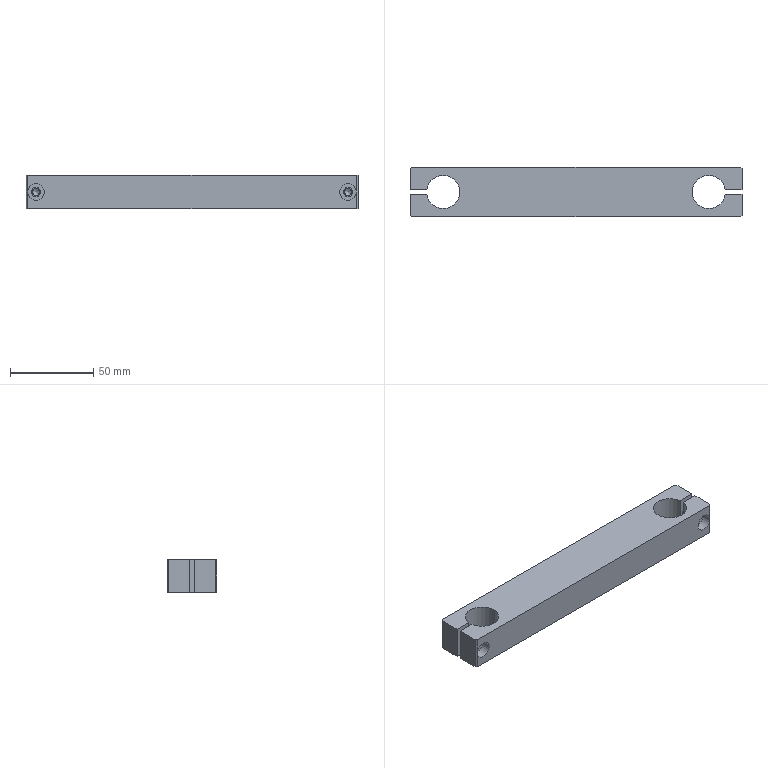Part | NX | features B0002 2 | 1 solid | 30 faces | box 200 x 30 x 20 mm | volume 103319 mm3 | plane 18 | cylinder 9 | cone 3 | commonest cylinder face diameters 4.2 x2 5.5 x2 10 x2 20 x2 8.5 x1
STEP:
#1=CARTESIAN_POINT('',(-94.,15.7,-379.25));
#2=VERTEX_POINT('',#1);
#3=CARTESIAN_POINT('',(-94.,15.7,-382.));
#4=DIRECTION('',(0.,1.,0.));
#5=DIRECTION('',(0.,0.,1.));
#6=AXIS2_PLACEMENT_3D('',#3,#4,#5);
#7=CIRCLE('',#6,2.75);
#8=EDGE_CURVE('',#2,#2,#7,.T.);
#9=ORIENTED_EDGE('',*,*,#8,.T.);
#10=EDGE_LOOP('',(#9));
#11=FACE_BOUND('',#10,.T.);
#12=CARTESIAN_POINT('',(-94.,15.7,-377.));
#13=VERTEX_POINT('',#12);
#14=CARTESIAN_POINT('',(-94.,15.7,-382.));
#15=DIRECTION('',(0.,-1.,0.));
#16=DIRECTION('',(0.,0.,1.));
#17=AXIS2_PLACEMENT_3D('',#14,#15,#16);
#18=CIRCLE('',#17,5.);
#19=EDGE_CURVE('',#13,#13,#18,.T.);
#20=ORIENTED_EDGE('',*,*,#19,.T.);
#21=EDGE_LOOP('',(#20));
#22=FACE_BOUND('',#21,.T.);
#23=CARTESIAN_POINT('',(-96.75,15.7,-382.));
#24=DIRECTION('',(0.,1.,0.));
#25=DIRECTION('',(0.,0.,-1.));
#26=AXIS2_PLACEMENT_3D('',#23,#24,#25);
#27=PLANE('',#26);
#28=ADVANCED_FACE('',(#11,#22),#27,.F.);
#29=CARTESIAN_POINT('',(-99.,10.,-382.));
#30=VERTEX_POINT('',#29);
#31=CARTESIAN_POINT('',(-94.,10.,-382.));
#32=DIRECTION('',(0.,1.,0.));
#33=DIRECTION('',(0.,0.,-1.));
#34=AXIS2_PLACEMENT_3D('',#31,#32,#33);
#35=CIRCLE('',#34,5.);
#36=EDGE_CURVE('',#30,#30,#35,.T.);
#37=ORIENTED_EDGE('',*,*,#36,.F.);
#38=EDGE_LOOP('',(#37));
#39=FACE_BOUND('',#38,.T.);
#40=ORIENTED_EDGE('',*,*,#19,.F.);
#41=EDGE_LOOP('',(#40));
#42=FACE_BOUND('',#41,.T.);
#43=CARTESIAN_POINT('',(-94.,10.,-382.));
#44=DIRECTION('',(0.,-1.,0.));
#45=DIRECTION('',(0.,0.,1.));
#46=AXIS2_PLACEMENT_3D('',#43,#44,#45);
#47=CYLINDRICAL_SURFACE('',#46,5.);
#48=ADVANCED_FACE('',(#39,#42),#47,.F.);
#49=CARTESIAN_POINT('',(99.,10.,-382.));
#50=VERTEX_POINT('',#49);
#51=CARTESIAN_POINT('',(94.,10.,-382.));
#52=DIRECTION('',(0.,1.,0.));
#53=DIRECTION('',(0.,0.,1.));
#54=AXIS2_PLACEMENT_3D('',#51,#52,#53);
#55=CIRCLE('',#54,5.);
#56=EDGE_CURVE('',#50,#50,#55,.T.);
#57=ORIENTED_EDGE('',*,*,#56,.F.);
#58=EDGE_LOOP('',(#57));
#59=FACE_BOUND('',#58,.T.);
#60=CARTESIAN_POINT('',(94.,15.7,-377.));
#61=VERTEX_POINT('',#60);
#62=CARTESIAN_POINT('',(94.,15.7,-382.));
#63=DIRECTION('',(0.,-1.,0.));
#64=DIRECTION('',(0.,0.,1.));
#65=AXIS2_PLACEMENT_3D('',#62,#63,#64);
#66=CIRCLE('',#65,5.);
#67=EDGE_CURVE('',#61,#61,#66,.T.);
#68=ORIENTED_EDGE('',*,*,#67,.F.);
#69=EDGE_LOOP('',(#68));
#70=FACE_BOUND('',#69,.T.);
#71=CARTESIAN_POINT('',(94.,10.,-382.));
#72=DIRECTION('',(0.,-1.,0.));
#73=DIRECTION('',(0.,0.,1.));
#74=AXIS2_PLACEMENT_3D('',#71,#72,#73);
#75=CYLINDRICAL_SURFACE('',#74,5.);
#76=ADVANCED_FACE('',(#59,#70),#75,.F.);
#77=CARTESIAN_POINT('',(94.,15.7,-384.75));
#78=VERTEX_POINT('',#77);
#79=CARTESIAN_POINT('',(94.,15.7,-382.));
#80=DIRECTION('',(0.,1.,0.));
#81=DIRECTION('',(0.,0.,-1.));
#82=AXIS2_PLACEMENT_3D('',#79,#80,#81);
#83=CIRCLE('',#82,2.75);
#84=EDGE_CURVE('',#78,#78,#83,.T.);
#85=ORIENTED_EDGE('',*,*,#84,.T.);
#86=EDGE_LOOP('',(#85));
#87=FACE_BOUND('',#86,.T.);
#88=ORIENTED_EDGE('',*,*,#67,.T.);
#89=EDGE_LOOP('',(#88));
#90=FACE_BOUND('',#89,.T.);
#91=CARTESIAN_POINT('',(91.25,15.7,-382.));
#92=DIRECTION('',(0.,1.,0.));
#93=DIRECTION('',(0.,0.,-1.));
#94=AXIS2_PLACEMENT_3D('',#91,#92,#93);
#95=PLANE('',#94);
#96=ADVANCED_FACE('',(#87,#90),#95,.F.);
#97=CARTESIAN_POINT('',(94.,23.75,-379.25));
#98=VERTEX_POINT('',#97);
#99=CARTESIAN_POINT('',(94.,23.75,-382.));
#100=DIRECTION('',(0.,-1.,0.));
#101=DIRECTION('',(0.,0.,1.));
#102=AXIS2_PLACEMENT_3D('',#99,#100,#101);
#103=CIRCLE('',#102,2.75);
#104=EDGE_CURVE('',#98,#98,#103,.T.);
#105=ORIENTED_EDGE('',*,*,#104,.F.);
#106=EDGE_LOOP('',(#105));
#107=FACE_BOUND('',#106,.T.);
#108=ORIENTED_EDGE('',*,*,#84,.F.);
#109=EDGE_LOOP('',(#108));
#110=FACE_BOUND('',#109,.T.);
#111=CARTESIAN_POINT('',(94.,10.,-382.));
#112=DIRECTION('',(0.,-1.,0.));
#113=DIRECTION('',(0.,0.,1.));
#114=AXIS2_PLACEMENT_3D('',#111,#112,#113);
#115=CYLINDRICAL_SURFACE('',#114,2.75);
#116=ADVANCED_FACE('',(#107,#110),#115,.F.);
#117=CARTESIAN_POINT('',(94.,38.65,-379.9));
#118=VERTEX_POINT('',#117);
#119=CARTESIAN_POINT('',(94.,38.65,-382.));
#120=DIRECTION('',(0.,-1.,0.));
#121=DIRECTION('',(0.,0.,1.));
#122=AXIS2_PLACEMENT_3D('',#119,#120,#121);
#123=CIRCLE('',#122,2.1);
#124=EDGE_CURVE('',#118,#118,#123,.T.);
#125=ORIENTED_EDGE('',*,*,#124,.T.);
#126=EDGE_LOOP('',(#125));
#127=FACE_BOUND('',#126,.T.);
#128=CARTESIAN_POINT('',(94.,39.912,-382.));
#129=VERTEX_POINT('',#128);
#130=VERTEX_LOOP('',#129);
#131=FACE_BOUND('',#130,.T.);
#132=CARTESIAN_POINT('',(94.,39.912,-382.));
#133=DIRECTION('',(0.,-1.,0.));
#134=DIRECTION('',(0.,0.,1.));
#135=AXIS2_PLACEMENT_3D('',#132,#133,#134);
#136=CONICAL_SURFACE('',#135,0.,1.03);
#137=ADVANCED_FACE('',(#127,#131),#136,.F.);
#138=CARTESIAN_POINT('',(94.,26.25,-384.1));
#139=VERTEX_POINT('',#138);
#140=CARTESIAN_POINT('',(94.,26.25,-382.));
#141=DIRECTION('',(0.,1.,0.));
#142=DIRECTION('',(0.,0.,-1.));
#143=AXIS2_PLACEMENT_3D('',#140,#141,#142);
#144=CIRCLE('',#143,2.1);
#145=EDGE_CURVE('',#139,#139,#144,.T.);
#146=ORIENTED_EDGE('',*,*,#145,.F.);
#147=EDGE_LOOP('',(#146));
#148=FACE_BOUND('',#147,.T.);
#149=ORIENTED_EDGE('',*,*,#124,.F.);
#150=EDGE_LOOP('',(#149));
#151=FACE_BOUND('',#150,.T.);
#152=CARTESIAN_POINT('',(94.,26.25,-382.));
#153=DIRECTION('',(0.,-1.,0.));
#154=DIRECTION('',(0.,0.,1.));
#155=AXIS2_PLACEMENT_3D('',#152,#153,#154);
#156=CYLINDRICAL_SURFACE('',#155,2.1);
#157=ADVANCED_FACE('',(#148,#151),#156,.F.);
#158=CARTESIAN_POINT('',(0.,12.946,-382.));
#159=VERTEX_POINT('',#158);
#160=VERTEX_LOOP('',#159);
#161=FACE_BOUND('',#160,.T.);
#162=CARTESIAN_POINT('',(0.,15.5,-386.25));
#163=VERTEX_POINT('',#162);
#164=CARTESIAN_POINT('',(0.,15.5,-382.));
#165=DIRECTION('',(0.,1.,0.));
#166=DIRECTION('',(0.,0.,-1.));
#167=AXIS2_PLACEMENT_3D('',#164,#165,#166);
#168=CIRCLE('',#167,4.25);
#169=EDGE_CURVE('',#163,#163,#168,.T.);
#170=ORIENTED_EDGE('',*,*,#169,.T.);
#171=EDGE_LOOP('',(#170));
#172=FACE_BOUND('',#171,.T.);
#173=CARTESIAN_POINT('',(0.,12.946,-382.));
#174=DIRECTION('',(0.,1.,0.));
#175=DIRECTION('',(0.,0.,-1.));
#176=AXIS2_PLACEMENT_3D('',#173,#174,#175);
#177=CONICAL_SURFACE('',#176,0.,1.03);
#178=ADVANCED_FACE('',(#161,#172),#177,.F.);
#179=ORIENTED_EDGE('',*,*,#169,.F.);
#180=EDGE_LOOP('',(#179));
#181=FACE_BOUND('',#180,.T.);
#182=CARTESIAN_POINT('',(0.,40.,-377.75));
#183=VERTEX_POINT('',#182);
#184=CARTESIAN_POINT('',(0.,40.,-382.));
#185=DIRECTION('',(0.,-1.,0.));
#186=DIRECTION('',(0.,0.,1.));
#187=AXIS2_PLACEMENT_3D('',#184,#185,#186);
#188=CIRCLE('',#187,4.25);
#189=EDGE_CURVE('',#183,#183,#188,.T.);
#190=ORIENTED_EDGE('',*,*,#189,.F.);
#191=EDGE_LOOP('',(#190));
#192=FACE_BOUND('',#191,.T.);
#193=CARTESIAN_POINT('',(0.,40.,-382.));
#194=DIRECTION('',(0.,1.,0.));
#195=DIRECTION('',(0.,0.,-1.));
#196=AXIS2_PLACEMENT_3D('',#193,#194,#195);
#197=CYLINDRICAL_SURFACE('',#196,4.25);
#198=ADVANCED_FACE('',(#181,#192),#197,.F.);
#199=CARTESIAN_POINT('',(-94.,38.65,-379.9));
#200=VERTEX_POINT('',#199);
#201=CARTESIAN_POINT('',(-94.,38.65,-382.));
#202=DIRECTION('',(0.,-1.,0.));
#203=DIRECTION('',(0.,0.,1.));
#204=AXIS2_PLACEMENT_3D('',#201,#202,#203);
#205=CIRCLE('',#204,2.1);
#206=EDGE_CURVE('',#200,#200,#205,.T.);
#207=ORIENTED_EDGE('',*,*,#206,.T.);
#208=EDGE_LOOP('',(#207));
#209=FACE_BOUND('',#208,.T.);
#210=CARTESIAN_POINT('',(-94.,39.912,-382.));
#211=VERTEX_POINT('',#210);
#212=VERTEX_LOOP('',#211);
#213=FACE_BOUND('',#212,.T.);
#214=CARTESIAN_POINT('',(-94.,39.912,-382.));
#215=DIRECTION('',(0.,-1.,0.));
#216=DIRECTION('',(0.,0.,1.));
#217=AXIS2_PLACEMENT_3D('',#214,#215,#216);
#218=CONICAL_SURFACE('',#217,0.,1.03);
#219=ADVANCED_FACE('',(#209,#213),#218,.F.);
#220=ORIENTED_EDGE('',*,*,#206,.F.);
#221=EDGE_LOOP('',(#220));
#222=FACE_BOUND('',#221,.T.);
#223=CARTESIAN_POINT('',(-94.,26.25,-384.1));
#224=VERTEX_POINT('',#223);
#225=CARTESIAN_POINT('',(-94.,26.25,-382.));
#226=DIRECTION('',(0.,1.,0.));
#227=DIRECTION('',(0.,0.,-1.));
#228=AXIS2_PLACEMENT_3D('',#225,#226,#227);
#229=CIRCLE('',#228,2.1);
#230=EDGE_CURVE('',#224,#224,#229,.T.);
#231=ORIENTED_EDGE('',*,*,#230,.F.);
#232=EDGE_LOOP('',(#231));
#233=FACE_BOUND('',#232,.T.);
#234=CARTESIAN_POINT('',(-94.,26.25,-382.));
#235=DIRECTION('',(0.,-1.,0.));
#236=DIRECTION('',(0.,0.,1.));
#237=AXIS2_PLACEMENT_3D('',#234,#235,#236);
#238=CYLINDRICAL_SURFACE('',#237,2.1);
#239=ADVANCED_FACE('',(#222,#233),#238,.F.);
#240=ORIENTED_EDGE('',*,*,#230,.T.);
#241=EDGE_LOOP('',(#240));
#242=FACE_BOUND('',#241,.T.);
#243=CARTESIAN_POINT('',(-89.922,26.25,-372.));
#244=VERTEX_POINT('',#243);
#245=CARTESIAN_POINT('',(-89.922,26.25,-392.));
#246=VERTEX_POINT('',#245);
#247=CARTESIAN_POINT('',(-89.922,26.25,-372.));
#248=DIRECTION('',(0.,0.,-1.));
#249=VECTOR('',#248,1000.);
#250=LINE('',#247,#249);
#251=EDGE_CURVE('',#244,#246,#250,.T.);
#252=ORIENTED_EDGE('',*,*,#251,.F.);
#253=CARTESIAN_POINT('',(-100.,26.25,-372.));
#254=VERTEX_POINT('',#253);
#255=CARTESIAN_POINT('',(-100.,26.25,-372.));
#256=DIRECTION('',(1.,0.,0.));
#257=VECTOR('',#256,1000.);
#258=LINE('',#255,#257);
#259=EDGE_CURVE('',#254,#244,#258,.T.);
#260=ORIENTED_EDGE('',*,*,#259,.F.);
#261=CARTESIAN_POINT('',(-100.,26.25,-392.));
#262=VERTEX_POINT('',#261);
#263=CARTESIAN_POINT('',(-100.,26.25,-372.));
#264=DIRECTION('',(0.,0.,-1.));
#265=VECTOR('',#264,1000.);
#266=LINE('',#263,#265);
#267=EDGE_CURVE('',#254,#262,#266,.T.);
#268=ORIENTED_EDGE('',*,*,#267,.T.);
#269=CARTESIAN_POINT('',(-89.922,26.25,-392.));
#270=DIRECTION('',(-1.,0.,0.));
#271=VECTOR('',#270,1000.);
#272=LINE('',#269,#271);
#273=EDGE_CURVE('',#246,#262,#272,.T.);
#274=ORIENTED_EDGE('',*,*,#273,.F.);
#275=EDGE_LOOP('',(#252,#260,#268,#274));
#276=FACE_BOUND('',#275,.T.);
#277=CARTESIAN_POINT('',(-80.,26.25,-392.001));
#278=DIRECTION('',(0.,1.,0.));
#279=DIRECTION('',(-1.,0.,0.));
#280=AXIS2_PLACEMENT_3D('',#277,#278,#279);
#281=PLANE('',#280);
#282=ADVANCED_FACE('',(#242,#276),#281,.F.);
#283=ORIENTED_EDGE('',*,*,#267,.F.);
#284=CARTESIAN_POINT('',(-100.,39.,-372.));
#285=VERTEX_POINT('',#284);
#286=CARTESIAN_POINT('',(-100.,26.25,-372.));
#287=DIRECTION('',(0.,1.,0.));
#288=VECTOR('',#287,1000.);
#289=LINE('',#286,#288);
#290=EDGE_CURVE('',#254,#285,#289,.T.);
#291=ORIENTED_EDGE('',*,*,#290,.T.);
#292=CARTESIAN_POINT('',(-100.,39.,-392.));
#293=VERTEX_POINT('',#292);
#294=CARTESIAN_POINT('',(-100.,39.,-392.));
#295=DIRECTION('',(0.,0.,1.));
#296=VECTOR('',#295,1000.);
#297=LINE('',#294,#296);
#298=EDGE_CURVE('',#293,#285,#297,.T.);
#299=ORIENTED_EDGE('',*,*,#298,.F.);
#300=CARTESIAN_POINT('',(-100.,26.25,-392.));
#301=DIRECTION('',(0.,1.,0.));
#302=VECTOR('',#301,1000.);
#303=LINE('',#300,#302);
#304=EDGE_CURVE('',#262,#293,#303,.T.);
#305=ORIENTED_EDGE('',*,*,#304,.F.);
#306=EDGE_LOOP('',(#283,#291,#299,#305));
#307=FACE_BOUND('',#306,.T.);
#308=CARTESIAN_POINT('',(-100.,40.,-372.));
#309=DIRECTION('',(1.,0.,0.));
#310=DIRECTION('',(0.,0.,1.));
#311=AXIS2_PLACEMENT_3D('',#308,#309,#310);
#312=PLANE('',#311);
#313=ADVANCED_FACE('',(#307),#312,.F.);
#314=CARTESIAN_POINT('',(-99.,40.,-372.));
#315=VERTEX_POINT('',#314);
#316=CARTESIAN_POINT('',(-99.,40.,-392.));
#317=VERTEX_POINT('',#316);
#318=CARTESIAN_POINT('',(-99.,40.,-372.));
#319=DIRECTION('',(0.,0.,-1.));
#320=VECTOR('',#319,1000.);
#321=LINE('',#318,#320);
#322=EDGE_CURVE('',#315,#317,#321,.T.);
#323=ORIENTED_EDGE('',*,*,#322,.T.);
#324=CARTESIAN_POINT('',(-100.,39.,-392.));
#325=DIRECTION('',(0.7071,0.7071,0.));
#326=VECTOR('',#325,1000.);
#327=LINE('',#324,#326);
#328=EDGE_CURVE('',#293,#317,#327,.T.);
#329=ORIENTED_EDGE('',*,*,#328,.F.);
#330=ORIENTED_EDGE('',*,*,#298,.T.);
#331=CARTESIAN_POINT('',(-99.,40.,-372.));
#332=DIRECTION('',(-0.7071,-0.7071,0.));
#333=VECTOR('',#332,1000.);
#334=LINE('',#331,#333);
#335=EDGE_CURVE('',#315,#285,#334,.T.);
#336=ORIENTED_EDGE('',*,*,#335,.F.);
#337=EDGE_LOOP('',(#323,#329,#330,#336));
#338=FACE_BOUND('',#337,.T.);
#339=CARTESIAN_POINT('',(-100.,39.,-372.));
#340=DIRECTION('',(0.7071,-0.7071,0.));
#341=DIRECTION('',(0.,0.,-1.));
#342=AXIS2_PLACEMENT_3D('',#339,#340,#341);
#343=PLANE('',#342);
#344=ADVANCED_FACE('',(#338),#343,.F.);
#345=ORIENTED_EDGE('',*,*,#189,.T.);
#346=EDGE_LOOP('',(#345));
#347=FACE_BOUND('',#346,.T.);
#348=ORIENTED_EDGE('',*,*,#322,.F.);
#349=CARTESIAN_POINT('',(99.,40.,-372.));
#350=VERTEX_POINT('',#349);
#351=CARTESIAN_POINT('',(-99.,40.,-372.));
#352=DIRECTION('',(1.,0.,0.));
#353=VECTOR('',#352,1000.);
#354=LINE('',#351,#353);
#355=EDGE_CURVE('',#315,#350,#354,.T.);
#356=ORIENTED_EDGE('',*,*,#355,.T.);
#357=CARTESIAN_POINT('',(99.,40.,-392.));
#358=VERTEX_POINT('',#357);
#359=CARTESIAN_POINT('',(99.,40.,-392.));
#360=DIRECTION('',(0.,0.,1.));
#361=VECTOR('',#360,1000.);
#362=LINE('',#359,#361);
#363=EDGE_CURVE('',#358,#350,#362,.T.);
#364=ORIENTED_EDGE('',*,*,#363,.F.);
#365=CARTESIAN_POINT('',(-99.,40.,-392.));
#366=DIRECTION('',(1.,0.,0.));
#367=VECTOR('',#366,1000.);
#368=LINE('',#365,#367);
#369=EDGE_CURVE('',#317,#358,#368,.T.);
#370=ORIENTED_EDGE('',*,*,#369,.F.);
#371=EDGE_LOOP('',(#348,#356,#364,#370));
#372=FACE_BOUND('',#371,.T.);
#373=CARTESIAN_POINT('',(-100.,40.,-372.));
#374=DIRECTION('',(0.,-1.,0.));
#375=DIRECTION('',(1.,0.,0.));
#376=AXIS2_PLACEMENT_3D('',#373,#374,#375);
#377=PLANE('',#376);
#378=ADVANCED_FACE('',(#347,#372),#377,.F.);
#379=CARTESIAN_POINT('',(100.,39.,-372.));
#380=VERTEX_POINT('',#379);
#381=CARTESIAN_POINT('',(100.,39.,-392.));
#382=VERTEX_POINT('',#381);
#383=CARTESIAN_POINT('',(100.,39.,-372.));
#384=DIRECTION('',(0.,0.,-1.));
#385=VECTOR('',#384,1000.);
#386=LINE('',#383,#385);
#387=EDGE_CURVE('',#380,#382,#386,.T.);
#388=ORIENTED_EDGE('',*,*,#387,.T.);
#389=CARTESIAN_POINT('',(99.,40.,-392.));
#390=DIRECTION('',(0.7071,-0.7071,0.));
#391=VECTOR('',#390,1000.);
#392=LINE('',#389,#391);
#393=EDGE_CURVE('',#358,#382,#392,.T.);
#394=ORIENTED_EDGE('',*,*,#393,.F.);
#395=ORIENTED_EDGE('',*,*,#363,.T.);
#396=CARTESIAN_POINT('',(100.,39.,-372.));
#397=DIRECTION('',(-0.7071,0.7071,0.));
#398=VECTOR('',#397,1000.);
#399=LINE('',#396,#398);
#400=EDGE_CURVE('',#380,#350,#399,.T.);
#401=ORIENTED_EDGE('',*,*,#400,.F.);
#402=EDGE_LOOP('',(#388,#394,#395,#401));
#403=FACE_BOUND('',#402,.T.);
#404=CARTESIAN_POINT('',(99.,40.,-372.));
#405=DIRECTION('',(-0.7071,-0.7071,0.));
#406=DIRECTION('',(0.,0.,-1.));
#407=AXIS2_PLACEMENT_3D('',#404,#405,#406);
#408=PLANE('',#407);
#409=ADVANCED_FACE('',(#403),#408,.F.);
#410=ORIENTED_EDGE('',*,*,#387,.F.);
#411=CARTESIAN_POINT('',(100.,26.25,-372.));
#412=VERTEX_POINT('',#411);
#413=CARTESIAN_POINT('',(100.,39.,-372.));
#414=DIRECTION('',(0.,-1.,0.));
#415=VECTOR('',#414,1000.);
#416=LINE('',#413,#415);
#417=EDGE_CURVE('',#380,#412,#416,.T.);
#418=ORIENTED_EDGE('',*,*,#417,.T.);
#419=CARTESIAN_POINT('',(100.,26.25,-392.));
#420=VERTEX_POINT('',#419);
#421=CARTESIAN_POINT('',(100.,26.25,-372.));
#422=DIRECTION('',(0.,0.,-1.));
#423=VECTOR('',#422,1000.);
#424=LINE('',#421,#423);
#425=EDGE_CURVE('',#412,#420,#424,.T.);
#426=ORIENTED_EDGE('',*,*,#425,.T.);
#427=CARTESIAN_POINT('',(100.,39.,-392.));
#428=DIRECTION('',(0.,-1.,0.));
#429=VECTOR('',#428,1000.);
#430=LINE('',#427,#429);
#431=EDGE_CURVE('',#382,#420,#430,.T.);
#432=ORIENTED_EDGE('',*,*,#431,.F.);
#433=EDGE_LOOP('',(#410,#418,#426,#432));
#434=FACE_BOUND('',#433,.T.);
#435=CARTESIAN_POINT('',(100.,40.,-372.));
#436=DIRECTION('',(-1.,0.,0.));
#437=DIRECTION('',(0.,0.,-1.));
#438=AXIS2_PLACEMENT_3D('',#435,#436,#437);
#439=PLANE('',#438);
#440=ADVANCED_FACE('',(#434),#439,.F.);
#441=ORIENTED_EDGE('',*,*,#145,.T.);
#442=EDGE_LOOP('',(#441));
#443=FACE_BOUND('',#442,.T.);
#444=CARTESIAN_POINT('',(89.922,26.25,-372.));
#445=VERTEX_POINT('',#444);
#446=CARTESIAN_POINT('',(100.,26.25,-372.));
#447=DIRECTION('',(-1.,0.,0.));
#448=VECTOR('',#447,1000.);
#449=LINE('',#446,#448);
#450=EDGE_CURVE('',#412,#445,#449,.T.);
#451=ORIENTED_EDGE('',*,*,#450,.T.);
#452=CARTESIAN_POINT('',(89.922,26.25,-392.));
#453=VERTEX_POINT('',#452);
#454=CARTESIAN_POINT('',(89.922,26.25,-392.));
#455=DIRECTION('',(0.,0.,1.));
#456=VECTOR('',#455,1000.);
#457=LINE('',#454,#456);
#458=EDGE_CURVE('',#453,#445,#457,.T.);
#459=ORIENTED_EDGE('',*,*,#458,.F.);
#460=CARTESIAN_POINT('',(89.922,26.25,-392.));
#461=DIRECTION('',(1.,0.,0.));
#462=VECTOR('',#461,1000.);
#463=LINE('',#460,#462);
#464=EDGE_CURVE('',#453,#420,#463,.T.);
#465=ORIENTED_EDGE('',*,*,#464,.T.);
#466=ORIENTED_EDGE('',*,*,#425,.F.);
#467=EDGE_LOOP('',(#451,#459,#465,#466));
#468=FACE_BOUND('',#467,.T.);
#469=CARTESIAN_POINT('',(80.,26.25,-392.001));
#470=DIRECTION('',(0.,-1.,0.));
#471=DIRECTION('',(1.,0.,0.));
#472=AXIS2_PLACEMENT_3D('',#469,#470,#471);
#473=PLANE('',#472);
#474=ADVANCED_FACE('',(#443,#468),#473,.T.);
#475=CARTESIAN_POINT('',(89.922,23.75,-392.));
#476=VERTEX_POINT('',#475);
#477=CARTESIAN_POINT('',(80.,25.,-392.));
#478=DIRECTION('',(0.,0.,1.));
#479=DIRECTION('',(0.9922,0.125,0.));
#480=AXIS2_PLACEMENT_3D('',#477,#478,#479);
#481=CIRCLE('',#480,10.);
#482=EDGE_CURVE('',#453,#476,#481,.T.);
#483=ORIENTED_EDGE('',*,*,#482,.F.);
#484=ORIENTED_EDGE('',*,*,#458,.T.);
#485=CARTESIAN_POINT('',(89.922,23.75,-372.));
#486=VERTEX_POINT('',#485);
#487=CARTESIAN_POINT('',(80.,25.,-372.));
#488=DIRECTION('',(0.,0.,-1.));
#489=DIRECTION('',(0.9922,-0.125,0.));
#490=AXIS2_PLACEMENT_3D('',#487,#488,#489);
#491=CIRCLE('',#490,10.);
#492=EDGE_CURVE('',#486,#445,#491,.T.);
#493=ORIENTED_EDGE('',*,*,#492,.F.);
#494=CARTESIAN_POINT('',(89.922,23.75,-372.));
#495=DIRECTION('',(0.,0.,-1.));
#496=VECTOR('',#495,1000.);
#497=LINE('',#494,#496);
#498=EDGE_CURVE('',#486,#476,#497,.T.);
#499=ORIENTED_EDGE('',*,*,#498,.T.);
#500=EDGE_LOOP('',(#483,#484,#493,#499));
#501=FACE_BOUND('',#500,.T.);
#502=CARTESIAN_POINT('',(80.,25.,-372.));
#503=DIRECTION('',(0.,0.,-1.));
#504=DIRECTION('',(1.,0.,0.));
#505=AXIS2_PLACEMENT_3D('',#502,#503,#504);
#506=CYLINDRICAL_SURFACE('',#505,10.);
#507=ADVANCED_FACE('',(#501),#506,.F.);
#508=ORIENTED_EDGE('',*,*,#104,.T.);
#509=EDGE_LOOP('',(#508));
#510=FACE_BOUND('',#509,.T.);
#511=ORIENTED_EDGE('',*,*,#498,.F.);
#512=CARTESIAN_POINT('',(100.,23.75,-372.));
#513=VERTEX_POINT('',#512);
#514=CARTESIAN_POINT('',(100.,23.75,-372.));
#515=DIRECTION('',(-1.,0.,0.));
#516=VECTOR('',#515,1000.);
#517=LINE('',#514,#516);
#518=EDGE_CURVE('',#513,#486,#517,.T.);
#519=ORIENTED_EDGE('',*,*,#518,.F.);
#520=CARTESIAN_POINT('',(100.,23.75,-392.));
#521=VERTEX_POINT('',#520);
#522=CARTESIAN_POINT('',(100.,23.75,-372.));
#523=DIRECTION('',(0.,0.,-1.));
#524=VECTOR('',#523,1000.);
#525=LINE('',#522,#524);
#526=EDGE_CURVE('',#513,#521,#525,.T.);
#527=ORIENTED_EDGE('',*,*,#526,.T.);
#528=CARTESIAN_POINT('',(89.922,23.75,-392.));
#529=DIRECTION('',(1.,0.,0.));
#530=VECTOR('',#529,1000.);
#531=LINE('',#528,#530);
#532=EDGE_CURVE('',#476,#521,#531,.T.);
#533=ORIENTED_EDGE('',*,*,#532,.F.);
#534=EDGE_LOOP('',(#511,#519,#527,#533));
#535=FACE_BOUND('',#534,.T.);
#536=CARTESIAN_POINT('',(80.,23.75,-392.001));
#537=DIRECTION('',(0.,-1.,0.));
#538=DIRECTION('',(1.,0.,0.));
#539=AXIS2_PLACEMENT_3D('',#536,#537,#538);
#540=PLANE('',#539);
#541=ADVANCED_FACE('',(#510,#535),#540,.F.);
#542=CARTESIAN_POINT('',(100.,11.,-392.));
#543=VERTEX_POINT('',#542);
#544=CARTESIAN_POINT('',(100.,11.,-372.));
#545=VERTEX_POINT('',#544);
#546=CARTESIAN_POINT('',(100.,11.,-392.));
#547=DIRECTION('',(0.,0.,1.));
#548=VECTOR('',#547,1000.);
#549=LINE('',#546,#548);
#550=EDGE_CURVE('',#543,#545,#549,.T.);
#551=ORIENTED_EDGE('',*,*,#550,.F.);
#552=CARTESIAN_POINT('',(100.,23.75,-392.));
#553=DIRECTION('',(0.,-1.,0.));
#554=VECTOR('',#553,1000.);
#555=LINE('',#552,#554);
#556=EDGE_CURVE('',#521,#543,#555,.T.);
#557=ORIENTED_EDGE('',*,*,#556,.F.);
#558=ORIENTED_EDGE('',*,*,#526,.F.);
#559=CARTESIAN_POINT('',(100.,23.75,-372.));
#560=DIRECTION('',(0.,-1.,0.));
#561=VECTOR('',#560,1000.);
#562=LINE('',#559,#561);
#563=EDGE_CURVE('',#513,#545,#562,.T.);
#564=ORIENTED_EDGE('',*,*,#563,.T.);
#565=EDGE_LOOP('',(#551,#557,#558,#564));
#566=FACE_BOUND('',#565,.T.);
#567=CARTESIAN_POINT('',(100.,40.,-372.));
#568=DIRECTION('',(-1.,0.,0.));
#569=DIRECTION('',(0.,0.,-1.));
#570=AXIS2_PLACEMENT_3D('',#567,#568,#569);
#571=PLANE('',#570);
#572=ADVANCED_FACE('',(#566),#571,.F.);
#573=CARTESIAN_POINT('',(99.,10.,-392.));
#574=VERTEX_POINT('',#573);
#575=CARTESIAN_POINT('',(99.,10.,-382.));
#576=DIRECTION('',(0.,0.,-1.));
#577=VECTOR('',#576,1000.);
#578=LINE('',#575,#577);
#579=EDGE_CURVE('',#50,#574,#578,.T.);
#580=ORIENTED_EDGE('',*,*,#579,.T.);
#581=CARTESIAN_POINT('',(100.,11.,-392.));
#582=DIRECTION('',(-0.7071,-0.7071,0.));
#583=VECTOR('',#582,1000.);
#584=LINE('',#581,#583);
#585=EDGE_CURVE('',#543,#574,#584,.T.);
#586=ORIENTED_EDGE('',*,*,#585,.F.);
#587=ORIENTED_EDGE('',*,*,#550,.T.);
#588=CARTESIAN_POINT('',(99.,10.,-372.));
#589=VERTEX_POINT('',#588);
#590=CARTESIAN_POINT('',(99.,10.,-372.));
#591=DIRECTION('',(0.7071,0.7071,0.));
#592=VECTOR('',#591,1000.);
#593=LINE('',#590,#592);
#594=EDGE_CURVE('',#589,#545,#593,.T.);
#595=ORIENTED_EDGE('',*,*,#594,.F.);
#596=CARTESIAN_POINT('',(99.,10.,-372.));
#597=DIRECTION('',(0.,0.,-1.));
#598=VECTOR('',#597,1000.);
#599=LINE('',#596,#598);
#600=EDGE_CURVE('',#589,#50,#599,.T.);
#601=ORIENTED_EDGE('',*,*,#600,.T.);
#602=EDGE_LOOP('',(#580,#586,#587,#595,#601));
#603=FACE_BOUND('',#602,.T.);
#604=CARTESIAN_POINT('',(100.,11.,-372.));
#605=DIRECTION('',(-0.7071,0.7071,0.));
#606=DIRECTION('',(0.,0.,-1.));
#607=AXIS2_PLACEMENT_3D('',#604,#605,#606);
#608=PLANE('',#607);
#609=ADVANCED_FACE('',(#603),#608,.F.);
#610=CARTESIAN_POINT('',(-99.,10.,-372.));
#611=VERTEX_POINT('',#610);
#612=CARTESIAN_POINT('',(-99.,10.,-382.));
#613=DIRECTION('',(0.,0.,1.));
#614=VECTOR('',#613,1000.);
#615=LINE('',#612,#614);
#616=EDGE_CURVE('',#30,#611,#615,.T.);
#617=ORIENTED_EDGE('',*,*,#616,.F.);
#618=ORIENTED_EDGE('',*,*,#36,.T.);
#619=CARTESIAN_POINT('',(-99.,10.,-392.));
#620=VERTEX_POINT('',#619);
#621=CARTESIAN_POINT('',(-99.,10.,-392.));
#622=DIRECTION('',(0.,0.,1.));
#623=VECTOR('',#622,1000.);
#624=LINE('',#621,#623);
#625=EDGE_CURVE('',#620,#30,#624,.T.);
#626=ORIENTED_EDGE('',*,*,#625,.F.);
#627=CARTESIAN_POINT('',(99.,10.,-392.));
#628=DIRECTION('',(-1.,0.,0.));
#629=VECTOR('',#628,1000.);
#630=LINE('',#627,#629);
#631=EDGE_CURVE('',#574,#620,#630,.T.);
#632=ORIENTED_EDGE('',*,*,#631,.F.);
#633=ORIENTED_EDGE('',*,*,#579,.F.);
#634=ORIENTED_EDGE('',*,*,#56,.T.);
#635=ORIENTED_EDGE('',*,*,#600,.F.);
#636=CARTESIAN_POINT('',(99.,10.,-372.));
#637=DIRECTION('',(-1.,0.,0.));
#638=VECTOR('',#637,1000.);
#639=LINE('',#636,#638);
#640=EDGE_CURVE('',#589,#611,#639,.T.);
#641=ORIENTED_EDGE('',*,*,#640,.T.);
#642=EDGE_LOOP('',(#617,#618,#626,#632,#633,#634,#635,#641));
#643=FACE_BOUND('',#642,.T.);
#644=CARTESIAN_POINT('',(-100.,10.,-372.));
#645=DIRECTION('',(0.,1.,0.));
#646=DIRECTION('',(-1.,0.,0.));
#647=AXIS2_PLACEMENT_3D('',#644,#645,#646);
#648=PLANE('',#647);
#649=ADVANCED_FACE('',(#643),#648,.F.);
#650=CARTESIAN_POINT('',(-100.,11.,-372.));
#651=VERTEX_POINT('',#650);
#652=CARTESIAN_POINT('',(-100.,11.,-392.));
#653=VERTEX_POINT('',#652);
#654=CARTESIAN_POINT('',(-100.,11.,-372.));
#655=DIRECTION('',(0.,0.,-1.));
#656=VECTOR('',#655,1000.);
#657=LINE('',#654,#656);
#658=EDGE_CURVE('',#651,#653,#657,.T.);
#659=ORIENTED_EDGE('',*,*,#658,.T.);
#660=CARTESIAN_POINT('',(-99.,10.,-392.));
#661=DIRECTION('',(-0.7071,0.7071,0.));
#662=VECTOR('',#661,1000.);
#663=LINE('',#660,#662);
#664=EDGE_CURVE('',#620,#653,#663,.T.);
#665=ORIENTED_EDGE('',*,*,#664,.F.);
#666=ORIENTED_EDGE('',*,*,#625,.T.);
#667=ORIENTED_EDGE('',*,*,#616,.T.);
#668=CARTESIAN_POINT('',(-100.,11.,-372.));
#669=DIRECTION('',(0.7071,-0.7071,0.));
#670=VECTOR('',#669,1000.);
#671=LINE('',#668,#670);
#672=EDGE_CURVE('',#651,#611,#671,.T.);
#673=ORIENTED_EDGE('',*,*,#672,.F.);
#674=EDGE_LOOP('',(#659,#665,#666,#667,#673));
#675=FACE_BOUND('',#674,.T.);
#676=CARTESIAN_POINT('',(-99.,10.,-372.));
#677=DIRECTION('',(0.7071,0.7071,0.));
#678=DIRECTION('',(0.,0.,-1.));
#679=AXIS2_PLACEMENT_3D('',#676,#677,#678);
#680=PLANE('',#679);
#681=ADVANCED_FACE('',(#675),#680,.F.);
#682=CARTESIAN_POINT('',(-89.922,23.75,-392.));
#683=VERTEX_POINT('',#682);
#684=CARTESIAN_POINT('',(-80.,25.,-392.));
#685=DIRECTION('',(0.,0.,1.));
#686=DIRECTION('',(-0.9922,-0.125,0.));
#687=AXIS2_PLACEMENT_3D('',#684,#685,#686);
#688=CIRCLE('',#687,10.);
#689=EDGE_CURVE('',#683,#246,#688,.T.);
#690=ORIENTED_EDGE('',*,*,#689,.T.);
#691=ORIENTED_EDGE('',*,*,#273,.T.);
#692=ORIENTED_EDGE('',*,*,#304,.T.);
#693=ORIENTED_EDGE('',*,*,#328,.T.);
#694=ORIENTED_EDGE('',*,*,#369,.T.);
#695=ORIENTED_EDGE('',*,*,#393,.T.);
#696=ORIENTED_EDGE('',*,*,#431,.T.);
#697=ORIENTED_EDGE('',*,*,#464,.F.);
#698=ORIENTED_EDGE('',*,*,#482,.T.);
#699=ORIENTED_EDGE('',*,*,#532,.T.);
#700=ORIENTED_EDGE('',*,*,#556,.T.);
#701=ORIENTED_EDGE('',*,*,#585,.T.);
#702=ORIENTED_EDGE('',*,*,#631,.T.);
#703=ORIENTED_EDGE('',*,*,#664,.T.);
#704=CARTESIAN_POINT('',(-100.,23.75,-392.));
#705=VERTEX_POINT('',#704);
#706=CARTESIAN_POINT('',(-100.,11.,-392.));
#707=DIRECTION('',(0.,1.,0.));
#708=VECTOR('',#707,1000.);
#709=LINE('',#706,#708);
#710=EDGE_CURVE('',#653,#705,#709,.T.);
#711=ORIENTED_EDGE('',*,*,#710,.T.);
#712=CARTESIAN_POINT('',(-89.922,23.75,-392.));
#713=DIRECTION('',(-1.,0.,0.));
#714=VECTOR('',#713,1000.);
#715=LINE('',#712,#714);
#716=EDGE_CURVE('',#683,#705,#715,.T.);
#717=ORIENTED_EDGE('',*,*,#716,.F.);
#718=EDGE_LOOP('',(#690,#691,#692,#693,#694,#695,#696,#697,#698,#699,#700,#701,#702,#703,#711,#717));
#719=FACE_BOUND('',#718,.T.);
#720=CARTESIAN_POINT('',(0.,25.,-392.));
#721=DIRECTION('',(0.,0.,1.));
#722=DIRECTION('',(-1.,0.,0.));
#723=AXIS2_PLACEMENT_3D('',#720,#721,#722);
#724=PLANE('',#723);
#725=ADVANCED_FACE('',(#719),#724,.F.);
#726=CARTESIAN_POINT('',(-89.922,23.75,-372.));
#727=VERTEX_POINT('',#726);
#728=CARTESIAN_POINT('',(-80.,25.,-372.));
#729=DIRECTION('',(0.,0.,-1.));
#730=DIRECTION('',(1.,0.,0.));
#731=AXIS2_PLACEMENT_3D('',#728,#729,#730);
#732=CIRCLE('',#731,10.);
#733=EDGE_CURVE('',#244,#727,#732,.T.);
#734=ORIENTED_EDGE('',*,*,#733,.F.);
#735=ORIENTED_EDGE('',*,*,#251,.T.);
#736=ORIENTED_EDGE('',*,*,#689,.F.);
#737=CARTESIAN_POINT('',(-89.922,23.75,-392.));
#738=DIRECTION('',(0.,0.,1.));
#739=VECTOR('',#738,1000.);
#740=LINE('',#737,#739);
#741=EDGE_CURVE('',#683,#727,#740,.T.);
#742=ORIENTED_EDGE('',*,*,#741,.T.);
#743=EDGE_LOOP('',(#734,#735,#736,#742));
#744=FACE_BOUND('',#743,.T.);
#745=CARTESIAN_POINT('',(-80.,25.,-372.));
#746=DIRECTION('',(0.,0.,-1.));
#747=DIRECTION('',(1.,0.,0.));
#748=AXIS2_PLACEMENT_3D('',#745,#746,#747);
#749=CYLINDRICAL_SURFACE('',#748,10.);
#750=ADVANCED_FACE('',(#744),#749,.F.);
#751=CARTESIAN_POINT('',(-100.,23.75,-372.));
#752=VERTEX_POINT('',#751);
#753=CARTESIAN_POINT('',(-100.,23.75,-372.));
#754=DIRECTION('',(1.,0.,0.));
#755=VECTOR('',#754,1000.);
#756=LINE('',#753,#755);
#757=EDGE_CURVE('',#752,#727,#756,.T.);
#758=ORIENTED_EDGE('',*,*,#757,.F.);
#759=CARTESIAN_POINT('',(-100.,11.,-372.));
#760=DIRECTION('',(0.,1.,0.));
#761=VECTOR('',#760,1000.);
#762=LINE('',#759,#761);
#763=EDGE_CURVE('',#651,#752,#762,.T.);
#764=ORIENTED_EDGE('',*,*,#763,.F.);
#765=ORIENTED_EDGE('',*,*,#672,.T.);
#766=ORIENTED_EDGE('',*,*,#640,.F.);
#767=ORIENTED_EDGE('',*,*,#594,.T.);
#768=ORIENTED_EDGE('',*,*,#563,.F.);
#769=ORIENTED_EDGE('',*,*,#518,.T.);
#770=ORIENTED_EDGE('',*,*,#492,.T.);
#771=ORIENTED_EDGE('',*,*,#450,.F.);
#772=ORIENTED_EDGE('',*,*,#417,.F.);
#773=ORIENTED_EDGE('',*,*,#400,.T.);
#774=ORIENTED_EDGE('',*,*,#355,.F.);
#775=ORIENTED_EDGE('',*,*,#335,.T.);
#776=ORIENTED_EDGE('',*,*,#290,.F.);
#777=ORIENTED_EDGE('',*,*,#259,.T.);
#778=ORIENTED_EDGE('',*,*,#733,.T.);
#779=EDGE_LOOP('',(#758,#764,#765,#766,#767,#768,#769,#770,#771,#772,#773,#774,#775,#776,#777,#778));
#780=FACE_BOUND('',#779,.T.);
#781=CARTESIAN_POINT('',(0.,25.,-372.));
#782=DIRECTION('',(0.,0.,1.));
#783=DIRECTION('',(-1.,0.,0.));
#784=AXIS2_PLACEMENT_3D('',#781,#782,#783);
#785=PLANE('',#784);
#786=ADVANCED_FACE('',(#780),#785,.T.);
#787=ORIENTED_EDGE('',*,*,#710,.F.);
#788=ORIENTED_EDGE('',*,*,#658,.F.);
#789=ORIENTED_EDGE('',*,*,#763,.T.);
#790=CARTESIAN_POINT('',(-100.,23.75,-372.));
#791=DIRECTION('',(0.,0.,-1.));
#792=VECTOR('',#791,1000.);
#793=LINE('',#790,#792);
#794=EDGE_CURVE('',#752,#705,#793,.T.);
#795=ORIENTED_EDGE('',*,*,#794,.T.);
#796=EDGE_LOOP('',(#787,#788,#789,#795));
#797=FACE_BOUND('',#796,.T.);
#798=CARTESIAN_POINT('',(-100.,40.,-372.));
#799=DIRECTION('',(1.,0.,0.));
#800=DIRECTION('',(0.,0.,1.));
#801=AXIS2_PLACEMENT_3D('',#798,#799,#800);
#802=PLANE('',#801);
#803=ADVANCED_FACE('',(#797),#802,.F.);
#804=CARTESIAN_POINT('',(-94.,23.75,-384.75));
#805=VERTEX_POINT('',#804);
#806=CARTESIAN_POINT('',(-94.,23.75,-382.));
#807=DIRECTION('',(0.,-1.,0.));
#808=DIRECTION('',(0.,0.,-1.));
#809=AXIS2_PLACEMENT_3D('',#806,#807,#808);
#810=CIRCLE('',#809,2.75);
#811=EDGE_CURVE('',#805,#805,#810,.T.);
#812=ORIENTED_EDGE('',*,*,#811,.T.);
#813=EDGE_LOOP('',(#812));
#814=FACE_BOUND('',#813,.T.);
#815=ORIENTED_EDGE('',*,*,#757,.T.);
#816=ORIENTED_EDGE('',*,*,#741,.F.);
#817=ORIENTED_EDGE('',*,*,#716,.T.);
#818=ORIENTED_EDGE('',*,*,#794,.F.);
#819=EDGE_LOOP('',(#815,#816,#817,#818));
#820=FACE_BOUND('',#819,.T.);
#821=CARTESIAN_POINT('',(-80.,23.75,-392.001));
#822=DIRECTION('',(0.,1.,0.));
#823=DIRECTION('',(-1.,0.,0.));
#824=AXIS2_PLACEMENT_3D('',#821,#822,#823);
#825=PLANE('',#824);
#826=ADVANCED_FACE('',(#814,#820),#825,.T.);
#827=ORIENTED_EDGE('',*,*,#811,.F.);
#828=EDGE_LOOP('',(#827));
#829=FACE_BOUND('',#828,.T.);
#830=ORIENTED_EDGE('',*,*,#8,.F.);
#831=EDGE_LOOP('',(#830));
#832=FACE_BOUND('',#831,.T.);
#833=CARTESIAN_POINT('',(-94.,10.,-382.));
#834=DIRECTION('',(0.,-1.,0.));
#835=DIRECTION('',(0.,0.,1.));
#836=AXIS2_PLACEMENT_3D('',#833,#834,#835);
#837=CYLINDRICAL_SURFACE('',#836,2.75);
#838=ADVANCED_FACE('',(#829,#832),#837,.F.);
#839=CLOSED_SHELL('',(#28,#48,#76,#96,#116,#137,#157,#178,#198,#219,#239,#282,#313,#344,#378,#409,#440,#474,#507,#541,#572,#609,#649,#681,#725,#750,#786,#803,#826,#838));
#840=MANIFOLD_SOLID_BREP('',#839);
#841=(LENGTH_UNIT()NAMED_UNIT(*)SI_UNIT(.MILLI.,.METRE.));
#842=UNCERTAINTY_MEASURE_WITH_UNIT(LENGTH_MEASURE(0.00001),#841,'','');
#843=(NAMED_UNIT(*)PLANE_ANGLE_UNIT()SI_UNIT($,.RADIAN.));
#844=(NAMED_UNIT(*)SI_UNIT($,.STERADIAN.)SOLID_ANGLE_UNIT());
#845=(GEOMETRIC_REPRESENTATION_CONTEXT(3)GLOBAL_UNCERTAINTY_ASSIGNED_CONTEXT((#842))GLOBAL_UNIT_ASSIGNED_CONTEXT((#841,#843,#844))REPRESENTATION_CONTEXT('',''));
#846=ADVANCED_BREP_SHAPE_REPRESENTATION('',(#840),#845);